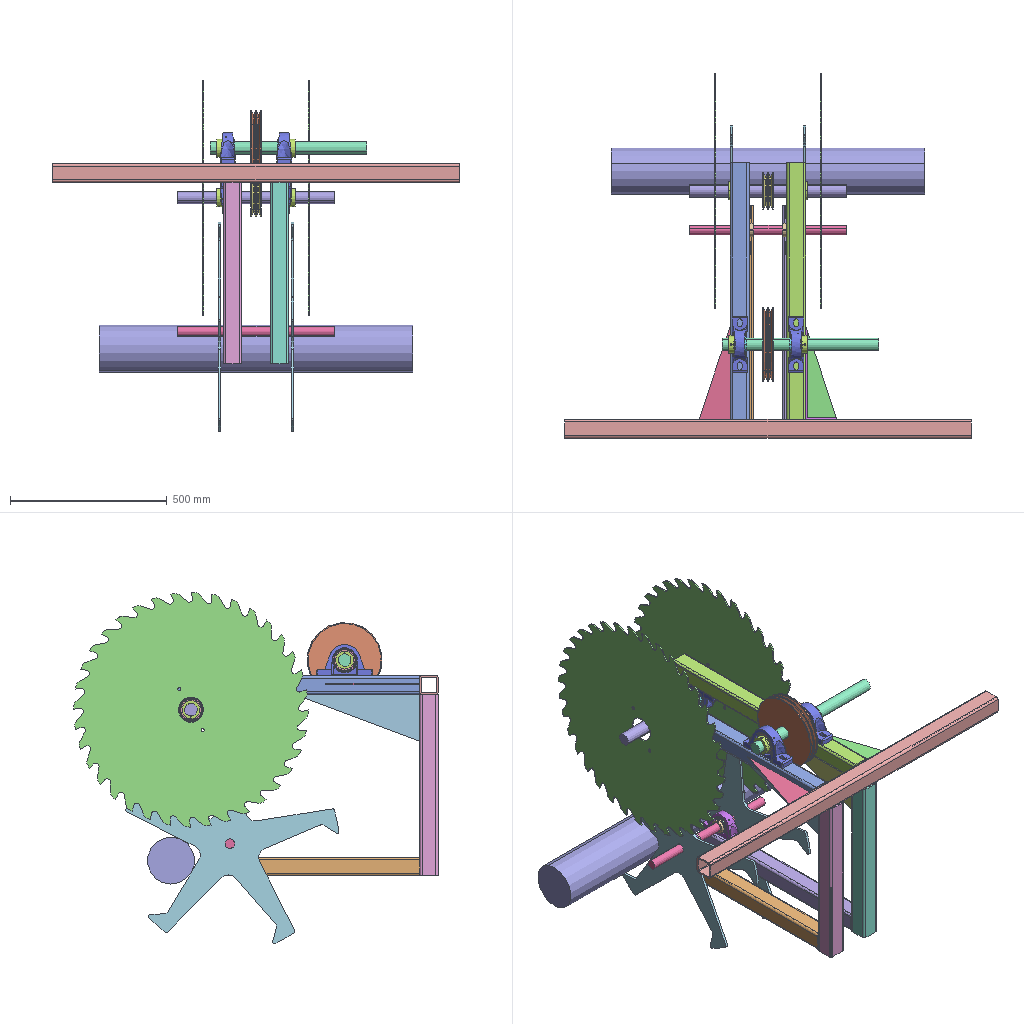Assembly | SolidWorks | 38 different items | 101 placed | box 1300 x 1165 x 1123 mm
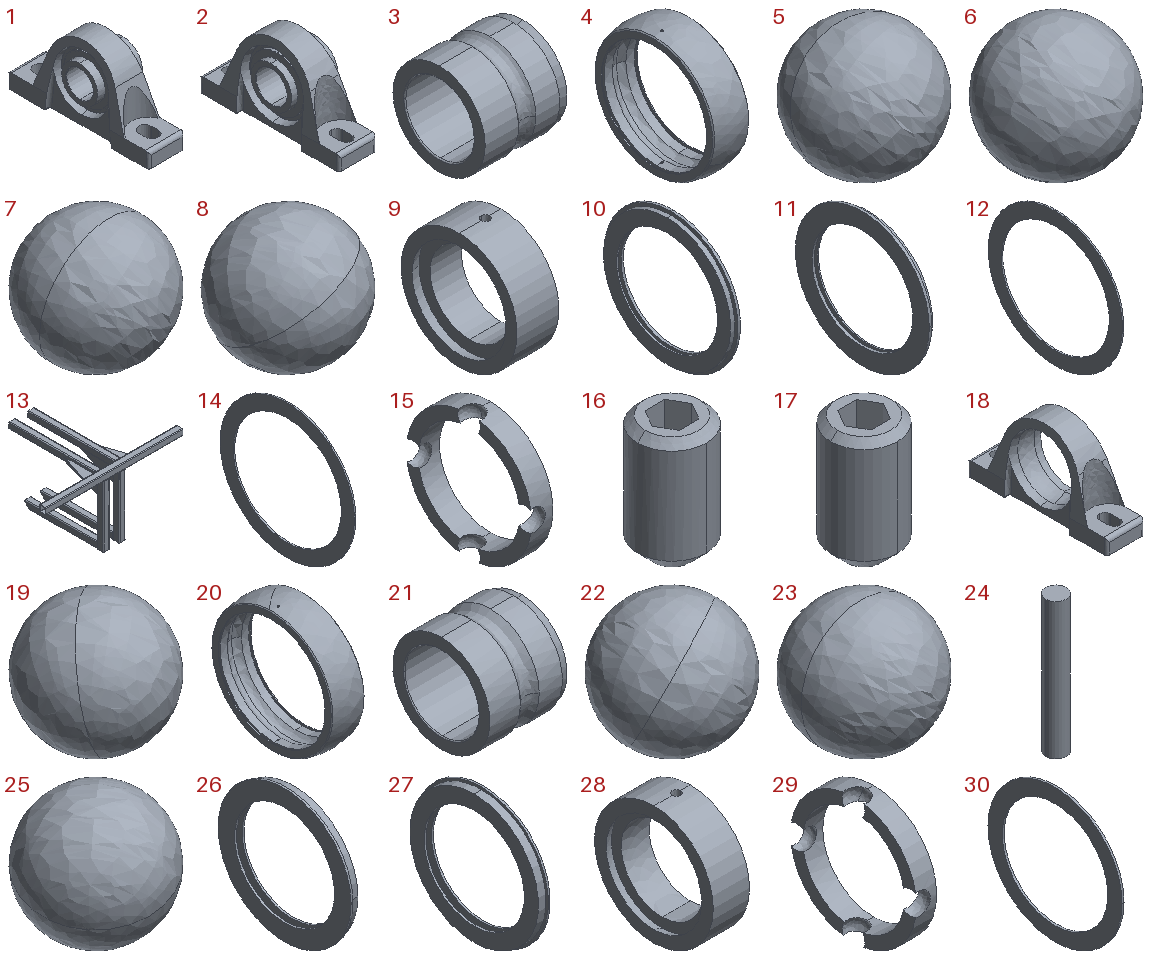Parts list (item | name | quantity | parent item | size | volume | features):
1 | (subassembly) | x2 | - | 50.1 x 158 x 82 mm | 190422 mm3 | -
2 | (subassembly) | x4 | - | 59.2 x 179 x 99 mm | 299518 mm3 | -
3 | - | x2 | in 1 | 36.5 x 40.2 x 40.2 mm | 18564 mm3 | features BaseBody 1
4 | - | x2 | in 1 | 18 x 62 x 62 mm | 12092 mm3 | features BaseBody 1
5 | - | x2 | in 1 | 9.525 x 9.525 x 9.525 mm | 452.463 mm3 | features BaseBody 1
6 | - | x2 | in 1 | 9.525 x 9.525 x 9.525 mm | 452.463 mm3 | features BaseBody 1
7 | - | x2 | in 1 | 9.525 x 9.525 x 9.525 mm | 452.463 mm3 | features BaseBody 1
8 | - | x2 | in 1 | 9.525 x 9.525 x 9.525 mm | 452.463 mm3 | features BaseBody 1
9 | - | x2 | in 1 | 15.9 x 44 x 44 mm | 11392 mm3 | features BaseBody 1
10 | - | x2 | in 1 | 2.7 x 54.668 x 54.668 mm | 1535 mm3 | features BaseBody 1
11 | - | x2 | in 1 | 2.7 x 54.668 x 54.668 mm | 1535 mm3 | features BaseBody 1
12 | - | x2 | in 1 | 0.54 x 50 x 50 mm | 374.901 mm3 | features BaseBody 1
13 | - | x1 | - | 1300 x 880 x 640 mm | 6179096 mm3 | features Gusset 4, WeldMemberFeat 3, WeldCornerFeat 2, ICE 1, WeldBeadFeat 1, WeldmentFeature 1
14 | - | x2 | in 1 | 0.54 x 50 x 50 mm | 374.901 mm3 | features BaseBody 1
15 | - | x2 | in 1 | 8.629 x 50.763 x 50.763 mm | 5071 mm3 | features BaseBody 1
16 | - | x2 | in 1 | 4 x 4 x 7 mm | 66.624 mm3 | features BaseBody 1
17 | - | x4 | in 2 | 5 x 5 x 9 mm | 134.698 mm3 | features BaseBody 1
18 | - | x4 | in 2 | 48 x 179 x 99 mm | 196943 mm3 | features BaseBody 1
19 | - | x4 | in 2 | 12.7 x 12.7 x 12.7 mm | 1073 mm3 | features BaseBody 1
20 | - | x4 | in 2 | 21 x 80 x 80 mm | 21730 mm3 | features BaseBody 1
21 | - | x4 | in 2 | 42.9 x 52.3 x 52.3 mm | 34134 mm3 | features BaseBody 1
22 | - | x4 | in 2 | 12.7 x 12.7 x 12.7 mm | 1073 mm3 | features BaseBody 1
23 | - | x4 | in 2 | 12.7 x 12.7 x 12.7 mm | 1073 mm3 | features BaseBody 1
24 | - | x1 | - | 150 x 150 x 1000 mm | 17671459 mm3 | features Extrusion 1
25 | - | x4 | in 2 | 12.7 x 12.7 x 12.7 mm | 1073 mm3 | features BaseBody 1
26 | - | x4 | in 2 | 4.95 x 70.89 x 70.89 mm | 3449 mm3 | features BaseBody 1
27 | - | x4 | in 2 | 4.95 x 70.89 x 70.89 mm | 3449 mm3 | features BaseBody 1
28 | - | x4 | in 2 | 17.7 x 58 x 58 mm | 22163 mm3 | features BaseBody 1
29 | - | x4 | in 2 | - | 10638 mm3 | features BaseBody 1
30 | - | x4 | in 2 | 0.99 x 66.3 x 66.3 mm | 1291 mm3 | features BaseBody 1
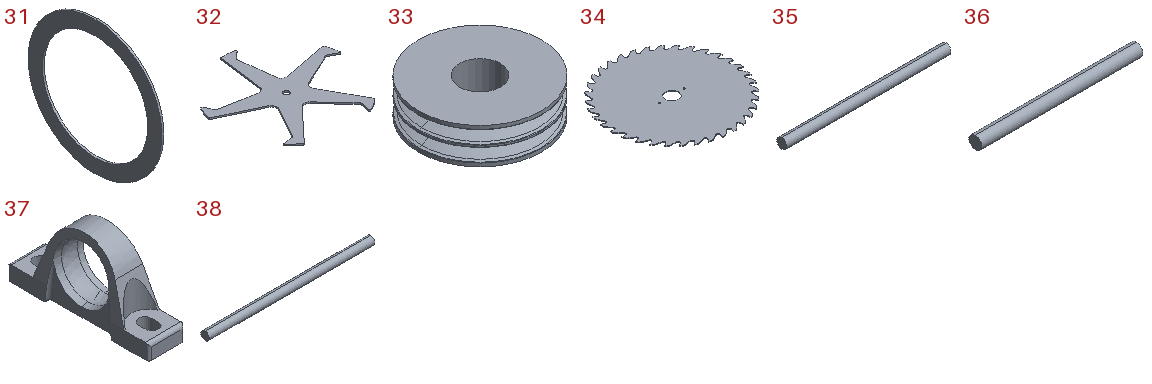31 | - | x4 | in 2 | 0.99 x 66.3 x 66.3 mm | 1291 mm3 | features BaseBody 1
32 | - | x2 | - | 682.923 x 664.717 x 8 mm | 939255 mm3 | features Extrusion 1
33 | - | x2 | - | 120 x 120 x 35 mm | 274896 mm3 | features Extrusion 1, Fillet 1, LPattern 1, RevCut 1
34 | - | x2 | - | 750 x 750 x 4 mm | 1607952 mm3 | features Cut 1, Extrusion 1
35 | - | x1 | - | 500 x 30 x 30 mm | 353429 mm3 | features Extrusion 1
36 | - | x1 | - | 500 x 40 x 40 mm | 628319 mm3 | features Extrusion 1
37 | - | x2 | in 1 | 40 x 158 x 82 mm | 137607 mm3 | features BaseBody 1
38 | - | x1 | - | 800 x 40 x 40 mm | 1005310 mm3 | features Extrusion 1
Mates (type | each side: item.copy, entity, surface, feature):
DistanceDim | 34.1 face plane Dicke | 34.2 face plane Dicke
DistanceDim | 32.1 face plane Linear austragen1 | 34.1 face plane Dicke
Coincident | 32.1 face plane Linear austragen1 | 32.2 face plane Linear austragen1
Concentric | 34.1 face cylinder Linear Cut Extrude1 | 34.2 face cylinder Linear Cut Extrude1 | 2 times
Concentric | 34.1 face cylinder Linear Cut Extrude1 | 36.1 face cylinder Length
Concentric | 36.1 face cylinder Length | 28.1 edge
Concentric | 32.1 face cylinder Linear austragen1 | 35.1 face cylinder Length
Concentric | 32.2 face cylinder Linear austragen1 | 35.1 face cylinder Length
Width | 36.1 face plane Length | 36.1 face plane Length | 34.2 face plane Dicke | 34.1 face plane Dicke
Coincident | 36.1 face plane Length | 35.1 face plane Length
Concentric | 36.1 face cylinder Length | 33.1 face cylinder Linear austragen1
Symmetric | 36.1 face plane Length | 36.1 face plane Length | assembly plane
Symmetric | 32.1 face plane Linear austragen1 | 32.2 face plane Linear austragen1 | assembly plane
Concentric | 35.1 face cylinder Length | 3.1 face cylinder inafag_lase30-n_155rtuoy243f148519ye0wsu7
Coincident | 13.1 face plane Strukturbauteil7 | 37.1 face plane inafag_lase30-n_155rtuoy243f148519ye0wsu7
Concentric | 35.1 face cylinder Length | 9.1 face cylinder inafag_lase30-n_155rtuoy243f148519ye0wsu7
Coincident | 37.2 face plane inafag_lase30-n_155rtuoy243f148519ye0wsu7 | 37.1 face plane inafag_lase30-n_155rtuoy243f148519ye0wsu7
Symmetric | 37.2 face plane inafag_lase30-n_155rtuoy243f148519ye0wsu7 | 37.1 face plane inafag_lase30-n_155rtuoy243f148519ye0wsu7 | assembly plane
Coincident | 13.1 face plane Linear Cut Extrude1 | 37.1 face plane inafag_lase30-n_155rtuoy243f148519ye0wsu7
Coincident | 18.1 face plane inafag_lase40-n_8bx0atzarjmwtw17x9v30eugc | 18.2 face plane inafag_lase40-n_8bx0atzarjmwtw17x9v30eugc | 2 times
Coincident | 13.1 face plane Strukturbauteil1 | 18.1 face plane inafag_lase40-n_8bx0atzarjmwtw17x9v30eugc
Symmetric | 18.1 face plane inafag_lase40-n_8bx0atzarjmwtw17x9v30eugc | 18.2 face plane inafag_lase40-n_8bx0atzarjmwtw17x9v30eugc | assembly plane
Coincident | 13.1 face plane Strukturbauteil1 | 18.3 face plane inafag_lase40-n_8bx0atzarjmwtw17x9v30eugc
Coincident | 13.1 face plane Strukturbauteil1 | 18.4 face plane inafag_lase40-n_8bx0atzarjmwtw17x9v30eugc
Coincident | 18.3 face plane inafag_lase40-n_8bx0atzarjmwtw17x9v30eugc | 18.4 face plane inafag_lase40-n_8bx0atzarjmwtw17x9v30eugc
Symmetric | 18.3 face plane inafag_lase40-n_8bx0atzarjmwtw17x9v30eugc | 18.4 face plane inafag_lase40-n_8bx0atzarjmwtw17x9v30eugc | assembly plane
Coincident | 18.3 axis | 38.1 axis
Concentric | 38.1 face cylinder Length | 33.2 face cylinder Linear austragen1
Symmetric | 33.2 face plane Linear austragen1 | 33.2 face plane Linear austragen1 | assembly plane
BeltDim | 33.1 face cylinder Revolved Cut1 | 33.2 face cylinder Lineares Muster1
DistanceDim | 18.4 face plane inafag_lase40-n_8bx0atzarjmwtw17x9v30eugc | 13.1 face plane Strukturbauteil1
Coincident | 13.1 face plane Strukturbauteil1 | 18.2 face plane inafag_lase40-n_8bx0atzarjmwtw17x9v30eugc
Symmetric | 33.1 face plane Linear austragen1 | 33.1 face plane Linear austragen1 | assembly plane
LinearCoupler | 36.1 face cylinder Length | 33.1 face plane Linear austragen1
UniversalJoint | 36.1 face cylinder Length | 34.1 face cylinder Linear Cut Extrude1
UniversalJoint | 33.1 face cylinder Linear austragen1 | 36.1 face cylinder Length
UniversalJoint | 38.1 face cylinder Length | 33.2 face cylinder Linear austragen1
DistanceDim | 38.1 face plane Length | 28.2 face plane inafag_lase40-n_8bx0atzarjmwtw17x9v30eugc
Width | 13.1 face plane Strukturbauteil1 | 13.1 face plane Strukturbauteil1 | 18.3 face plane inafag_lase40-n_8bx0atzarjmwtw17x9v30eugc | 18.3 face plane inafag_lase40-n_8bx0atzarjmwtw17x9v30eugc
Tangent | 32.1 face plane Linear austragen1 | 24.1 face cylinder Length
Symmetric | 24.1 face plane Length | 24.1 face plane Length | assembly plane
Tangent | 32.2 face plane Linear austragen1 | 24.1 face cylinder Length